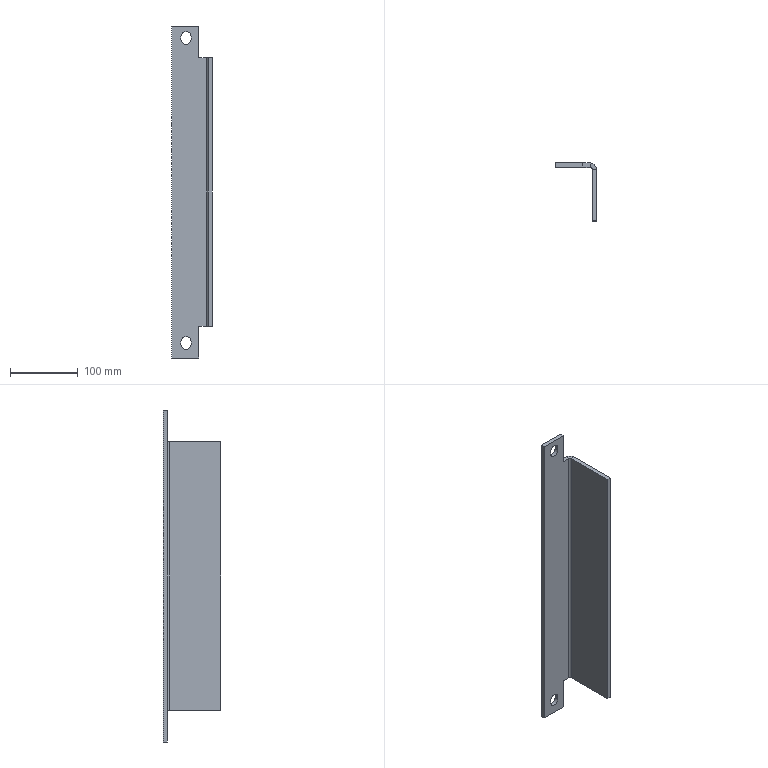Part | SolidWorks | features ICE 2, FlatPattern 1, SMBaseFlange 1, SheetMetal 1 | 1 solid | 28 faces | box 60 x 85 x 490 mm | volume 343865 mm3 | plane 20 | cylinder 8 | commonest cylinder face diameters 15 x6 6 x1 18 x1
STEP:
#1=CARTESIAN_POINT('',(-38.8,-6.,-213.5));
#2=VERTEX_POINT('',#1);
#3=CARTESIAN_POINT('',(-31.3,-6.,-221.));
#4=VERTEX_POINT('',#3);
#5=CARTESIAN_POINT('',(-38.8,-6.,-221.));
#6=DIRECTION('',(0.,1.,0.));
#7=DIRECTION('',(-1.,0.,0.));
#8=AXIS2_PLACEMENT_3D('',#5,#6,#7);
#9=CIRCLE('',#8,7.5);
#10=EDGE_CURVE('',#2,#4,#9,.T.);
#11=ORIENTED_EDGE('',*,*,#10,.F.);
#12=CARTESIAN_POINT('',(-38.8,0.,-213.5));
#13=VERTEX_POINT('',#12);
#14=CARTESIAN_POINT('',(-38.8,-85.,-213.5));
#15=DIRECTION('',(0.,1.,0.));
#16=VECTOR('',#15,1000.);
#17=LINE('',#14,#16);
#18=EDGE_CURVE('',#2,#13,#17,.T.);
#19=ORIENTED_EDGE('',*,*,#18,.T.);
#20=CARTESIAN_POINT('',(-31.3,0.,-221.));
#21=VERTEX_POINT('',#20);
#22=CARTESIAN_POINT('',(-38.8,0.,-221.));
#23=DIRECTION('',(0.,1.,0.));
#24=DIRECTION('',(0.,0.,1.));
#25=AXIS2_PLACEMENT_3D('',#22,#23,#24);
#26=CIRCLE('',#25,7.5);
#27=EDGE_CURVE('',#13,#21,#26,.T.);
#28=ORIENTED_EDGE('',*,*,#27,.T.);
#29=CARTESIAN_POINT('',(-31.3,-85.,-221.));
#30=DIRECTION('',(0.,1.,0.));
#31=VECTOR('',#30,1000.);
#32=LINE('',#29,#31);
#33=EDGE_CURVE('',#4,#21,#32,.T.);
#34=ORIENTED_EDGE('',*,*,#33,.F.);
#35=EDGE_LOOP('',(#11,#19,#28,#34));
#36=FACE_OUTER_BOUND('',#35,.T.);
#37=CARTESIAN_POINT('',(-38.8,-85.,-221.));
#38=DIRECTION('',(0.,1.,0.));
#39=DIRECTION('',(0.,0.,1.));
#40=AXIS2_PLACEMENT_3D('',#37,#38,#39);
#41=CYLINDRICAL_SURFACE('',#40,7.5);
#42=ADVANCED_FACE('',(#36),#41,.F.);
#43=CARTESIAN_POINT('',(-38.8,-6.,236.5));
#44=VERTEX_POINT('',#43);
#45=CARTESIAN_POINT('',(-31.3,-6.,229.));
#46=VERTEX_POINT('',#45);
#47=CARTESIAN_POINT('',(-38.8,-6.,229.));
#48=DIRECTION('',(0.,1.,0.));
#49=DIRECTION('',(-1.,0.,0.));
#50=AXIS2_PLACEMENT_3D('',#47,#48,#49);
#51=CIRCLE('',#50,7.5);
#52=EDGE_CURVE('',#44,#46,#51,.T.);
#53=ORIENTED_EDGE('',*,*,#52,.F.);
#54=CARTESIAN_POINT('',(-38.8,0.,236.5));
#55=VERTEX_POINT('',#54);
#56=CARTESIAN_POINT('',(-38.8,-85.,236.5));
#57=DIRECTION('',(0.,1.,0.));
#58=VECTOR('',#57,1000.);
#59=LINE('',#56,#58);
#60=EDGE_CURVE('',#44,#55,#59,.T.);
#61=ORIENTED_EDGE('',*,*,#60,.T.);
#62=CARTESIAN_POINT('',(-31.3,0.,229.));
#63=VERTEX_POINT('',#62);
#64=CARTESIAN_POINT('',(-38.8,0.,229.));
#65=DIRECTION('',(0.,1.,0.));
#66=DIRECTION('',(0.,0.,1.));
#67=AXIS2_PLACEMENT_3D('',#64,#65,#66);
#68=CIRCLE('',#67,7.5);
#69=EDGE_CURVE('',#55,#63,#68,.T.);
#70=ORIENTED_EDGE('',*,*,#69,.T.);
#71=CARTESIAN_POINT('',(-31.3,-85.,229.));
#72=DIRECTION('',(0.,1.,0.));
#73=VECTOR('',#72,1000.);
#74=LINE('',#71,#73);
#75=EDGE_CURVE('',#46,#63,#74,.T.);
#76=ORIENTED_EDGE('',*,*,#75,.F.);
#77=EDGE_LOOP('',(#53,#61,#70,#76));
#78=FACE_OUTER_BOUND('',#77,.T.);
#79=CARTESIAN_POINT('',(-38.8,-85.,229.));
#80=DIRECTION('',(0.,1.,0.));
#81=DIRECTION('',(0.,0.,1.));
#82=AXIS2_PLACEMENT_3D('',#79,#80,#81);
#83=CYLINDRICAL_SURFACE('',#82,7.5);
#84=ADVANCED_FACE('',(#78),#83,.F.);
#85=CARTESIAN_POINT('',(-6.,-9.,-198.));
#86=VERTEX_POINT('',#85);
#87=CARTESIAN_POINT('',(-6.,-85.,-198.));
#88=VERTEX_POINT('',#87);
#89=CARTESIAN_POINT('',(-6.,0.,-198.));
#90=DIRECTION('',(0.,-1.,0.));
#91=VECTOR('',#90,1000.);
#92=LINE('',#89,#91);
#93=EDGE_CURVE('',#86,#88,#92,.T.);
#94=ORIENTED_EDGE('',*,*,#93,.F.);
#95=CARTESIAN_POINT('',(0.,-9.,-198.));
#96=VERTEX_POINT('',#95);
#97=CARTESIAN_POINT('',(-6.,-9.,-198.));
#98=DIRECTION('',(1.,0.,0.));
#99=VECTOR('',#98,1000.);
#100=LINE('',#97,#99);
#101=EDGE_CURVE('',#86,#96,#100,.T.);
#102=ORIENTED_EDGE('',*,*,#101,.T.);
#103=CARTESIAN_POINT('',(0.,-85.,-198.));
#104=VERTEX_POINT('',#103);
#105=CARTESIAN_POINT('',(0.,-85.,-198.));
#106=DIRECTION('',(0.,-1.,0.));
#107=VECTOR('',#106,1000.);
#108=LINE('',#105,#107);
#109=EDGE_CURVE('',#96,#104,#108,.T.);
#110=ORIENTED_EDGE('',*,*,#109,.T.);
#111=CARTESIAN_POINT('',(-20.,-85.,-198.));
#112=DIRECTION('',(1.,0.,0.));
#113=VECTOR('',#112,1000.);
#114=LINE('',#111,#113);
#115=EDGE_CURVE('',#88,#104,#114,.T.);
#116=ORIENTED_EDGE('',*,*,#115,.F.);
#117=EDGE_LOOP('',(#94,#102,#110,#116));
#118=FACE_OUTER_BOUND('',#117,.T.);
#119=CARTESIAN_POINT('',(-20.,-85.,-198.));
#120=DIRECTION('',(0.,0.,1.));
#121=DIRECTION('',(1.,0.,0.));
#122=AXIS2_PLACEMENT_3D('',#119,#120,#121);
#123=PLANE('',#122);
#124=ADVANCED_FACE('',(#118),#123,.F.);
#125=CARTESIAN_POINT('',(-20.,0.,-198.));
#126=VERTEX_POINT('',#125);
#127=CARTESIAN_POINT('',(-9.,0.,-198.));
#128=VERTEX_POINT('',#127);
#129=CARTESIAN_POINT('',(-20.,0.,-198.));
#130=DIRECTION('',(1.,0.,0.));
#131=VECTOR('',#130,1000.);
#132=LINE('',#129,#131);
#133=EDGE_CURVE('',#126,#128,#132,.T.);
#134=ORIENTED_EDGE('',*,*,#133,.T.);
#135=CARTESIAN_POINT('',(-9.,-6.,-198.));
#136=VERTEX_POINT('',#135);
#137=CARTESIAN_POINT('',(-9.,0.,-198.));
#138=DIRECTION('',(0.,-1.,0.));
#139=VECTOR('',#138,1000.);
#140=LINE('',#137,#139);
#141=EDGE_CURVE('',#128,#136,#140,.T.);
#142=ORIENTED_EDGE('',*,*,#141,.T.);
#143=CARTESIAN_POINT('',(-20.,-6.,-198.));
#144=VERTEX_POINT('',#143);
#145=CARTESIAN_POINT('',(0.,-6.,-198.));
#146=DIRECTION('',(1.,0.,0.));
#147=VECTOR('',#146,1000.);
#148=LINE('',#145,#147);
#149=EDGE_CURVE('',#144,#136,#148,.T.);
#150=ORIENTED_EDGE('',*,*,#149,.F.);
#151=CARTESIAN_POINT('',(-20.,-85.,-198.));
#152=DIRECTION('',(0.,-1.,0.));
#153=VECTOR('',#152,1000.);
#154=LINE('',#151,#153);
#155=EDGE_CURVE('',#126,#144,#154,.T.);
#156=ORIENTED_EDGE('',*,*,#155,.F.);
#157=EDGE_LOOP('',(#134,#142,#150,#156));
#158=FACE_OUTER_BOUND('',#157,.T.);
#159=CARTESIAN_POINT('',(-20.,-85.,-198.));
#160=DIRECTION('',(0.,0.,1.));
#161=DIRECTION('',(1.,0.,0.));
#162=AXIS2_PLACEMENT_3D('',#159,#160,#161);
#163=PLANE('',#162);
#164=ADVANCED_FACE('',(#158),#163,.F.);
#165=CARTESIAN_POINT('',(-9.,-6.,198.));
#166=VERTEX_POINT('',#165);
#167=CARTESIAN_POINT('',(-20.,-6.,198.));
#168=VERTEX_POINT('',#167);
#169=CARTESIAN_POINT('',(0.,-6.,198.));
#170=DIRECTION('',(-1.,0.,0.));
#171=VECTOR('',#170,1000.);
#172=LINE('',#169,#171);
#173=EDGE_CURVE('',#166,#168,#172,.T.);
#174=ORIENTED_EDGE('',*,*,#173,.F.);
#175=CARTESIAN_POINT('',(-9.,0.,198.));
#176=VERTEX_POINT('',#175);
#177=CARTESIAN_POINT('',(-9.,-6.,198.));
#178=DIRECTION('',(0.,1.,0.));
#179=VECTOR('',#178,1000.);
#180=LINE('',#177,#179);
#181=EDGE_CURVE('',#166,#176,#180,.T.);
#182=ORIENTED_EDGE('',*,*,#181,.T.);
#183=CARTESIAN_POINT('',(-20.,0.,198.));
#184=VERTEX_POINT('',#183);
#185=CARTESIAN_POINT('',(-20.,0.,198.));
#186=DIRECTION('',(1.,0.,0.));
#187=VECTOR('',#186,1000.);
#188=LINE('',#185,#187);
#189=EDGE_CURVE('',#184,#176,#188,.T.);
#190=ORIENTED_EDGE('',*,*,#189,.F.);
#191=CARTESIAN_POINT('',(-20.,-85.,198.));
#192=DIRECTION('',(0.,1.,0.));
#193=VECTOR('',#192,1000.);
#194=LINE('',#191,#193);
#195=EDGE_CURVE('',#168,#184,#194,.T.);
#196=ORIENTED_EDGE('',*,*,#195,.F.);
#197=EDGE_LOOP('',(#174,#182,#190,#196));
#198=FACE_OUTER_BOUND('',#197,.T.);
#199=CARTESIAN_POINT('',(-20.,-85.,198.));
#200=DIRECTION('',(0.,0.,-1.));
#201=DIRECTION('',(-1.,0.,0.));
#202=AXIS2_PLACEMENT_3D('',#199,#200,#201);
#203=PLANE('',#202);
#204=ADVANCED_FACE('',(#198),#203,.F.);
#205=CARTESIAN_POINT('',(0.,-85.,198.));
#206=VERTEX_POINT('',#205);
#207=CARTESIAN_POINT('',(0.,-9.,198.));
#208=VERTEX_POINT('',#207);
#209=CARTESIAN_POINT('',(0.,-85.,198.));
#210=DIRECTION('',(0.,1.,0.));
#211=VECTOR('',#210,1000.);
#212=LINE('',#209,#211);
#213=EDGE_CURVE('',#206,#208,#212,.T.);
#214=ORIENTED_EDGE('',*,*,#213,.T.);
#215=CARTESIAN_POINT('',(-6.,-9.,198.));
#216=VERTEX_POINT('',#215);
#217=CARTESIAN_POINT('',(0.,-9.,198.));
#218=DIRECTION('',(-1.,0.,0.));
#219=VECTOR('',#218,1000.);
#220=LINE('',#217,#219);
#221=EDGE_CURVE('',#208,#216,#220,.T.);
#222=ORIENTED_EDGE('',*,*,#221,.T.);
#223=CARTESIAN_POINT('',(-6.,-85.,198.));
#224=VERTEX_POINT('',#223);
#225=CARTESIAN_POINT('',(-6.,0.,198.));
#226=DIRECTION('',(0.,1.,0.));
#227=VECTOR('',#226,1000.);
#228=LINE('',#225,#227);
#229=EDGE_CURVE('',#224,#216,#228,.T.);
#230=ORIENTED_EDGE('',*,*,#229,.F.);
#231=CARTESIAN_POINT('',(-20.,-85.,198.));
#232=DIRECTION('',(1.,0.,0.));
#233=VECTOR('',#232,1000.);
#234=LINE('',#231,#233);
#235=EDGE_CURVE('',#224,#206,#234,.T.);
#236=ORIENTED_EDGE('',*,*,#235,.T.);
#237=EDGE_LOOP('',(#214,#222,#230,#236));
#238=FACE_OUTER_BOUND('',#237,.T.);
#239=CARTESIAN_POINT('',(-20.,-85.,198.));
#240=DIRECTION('',(0.,0.,-1.));
#241=DIRECTION('',(-1.,0.,0.));
#242=AXIS2_PLACEMENT_3D('',#239,#240,#241);
#243=PLANE('',#242);
#244=ADVANCED_FACE('',(#238),#243,.F.);
#245=CARTESIAN_POINT('',(-20.,-6.,-245.));
#246=VERTEX_POINT('',#245);
#247=CARTESIAN_POINT('',(-20.,0.,-245.));
#248=VERTEX_POINT('',#247);
#249=CARTESIAN_POINT('',(-20.,-85.,-245.));
#250=DIRECTION('',(0.,1.,0.));
#251=VECTOR('',#250,1000.);
#252=LINE('',#249,#251);
#253=EDGE_CURVE('',#246,#248,#252,.T.);
#254=ORIENTED_EDGE('',*,*,#253,.F.);
#255=CARTESIAN_POINT('',(-60.,-6.,-245.));
#256=VERTEX_POINT('',#255);
#257=CARTESIAN_POINT('',(0.,-6.,-245.));
#258=DIRECTION('',(1.,0.,0.));
#259=VECTOR('',#258,1000.);
#260=LINE('',#257,#259);
#261=EDGE_CURVE('',#256,#246,#260,.T.);
#262=ORIENTED_EDGE('',*,*,#261,.F.);
#263=CARTESIAN_POINT('',(-60.,0.,-245.));
#264=VERTEX_POINT('',#263);
#265=CARTESIAN_POINT('',(-60.,-6.,-245.));
#266=DIRECTION('',(0.,1.,0.));
#267=VECTOR('',#266,1000.);
#268=LINE('',#265,#267);
#269=EDGE_CURVE('',#256,#264,#268,.T.);
#270=ORIENTED_EDGE('',*,*,#269,.T.);
#271=CARTESIAN_POINT('',(0.,0.,-245.));
#272=DIRECTION('',(1.,0.,0.));
#273=VECTOR('',#272,1000.);
#274=LINE('',#271,#273);
#275=EDGE_CURVE('',#264,#248,#274,.T.);
#276=ORIENTED_EDGE('',*,*,#275,.T.);
#277=EDGE_LOOP('',(#254,#262,#270,#276));
#278=FACE_OUTER_BOUND('',#277,.T.);
#279=CARTESIAN_POINT('',(-6.,-9.,-245.));
#280=DIRECTION('',(0.,0.,-1.));
#281=DIRECTION('',(-1.,0.,0.));
#282=AXIS2_PLACEMENT_3D('',#279,#280,#281);
#283=PLANE('',#282);
#284=ADVANCED_FACE('',(#278),#283,.T.);
#285=CARTESIAN_POINT('',(-6.,-85.,245.));
#286=DIRECTION('',(0.,0.,-1.));
#287=VECTOR('',#286,1000.);
#288=LINE('',#285,#287);
#289=EDGE_CURVE('',#224,#88,#288,.T.);
#290=ORIENTED_EDGE('',*,*,#289,.F.);
#291=ORIENTED_EDGE('',*,*,#229,.T.);
#292=CARTESIAN_POINT('',(-6.,-9.,245.));
#293=DIRECTION('',(0.,0.,-1.));
#294=VECTOR('',#293,1000.);
#295=LINE('',#292,#294);
#296=EDGE_CURVE('',#216,#86,#295,.T.);
#297=ORIENTED_EDGE('',*,*,#296,.T.);
#298=ORIENTED_EDGE('',*,*,#93,.T.);
#299=EDGE_LOOP('',(#290,#291,#297,#298));
#300=FACE_OUTER_BOUND('',#299,.T.);
#301=CARTESIAN_POINT('',(-6.,0.,245.));
#302=DIRECTION('',(1.,0.,0.));
#303=DIRECTION('',(0.,1.,0.));
#304=AXIS2_PLACEMENT_3D('',#301,#302,#303);
#305=PLANE('',#304);
#306=ADVANCED_FACE('',(#300),#305,.F.);
#307=ORIENTED_EDGE('',*,*,#235,.F.);
#308=ORIENTED_EDGE('',*,*,#289,.T.);
#309=ORIENTED_EDGE('',*,*,#115,.T.);
#310=CARTESIAN_POINT('',(0.,-85.,245.));
#311=DIRECTION('',(0.,0.,-1.));
#312=VECTOR('',#311,1000.);
#313=LINE('',#310,#312);
#314=EDGE_CURVE('',#206,#104,#313,.T.);
#315=ORIENTED_EDGE('',*,*,#314,.F.);
#316=EDGE_LOOP('',(#307,#308,#309,#315));
#317=FACE_OUTER_BOUND('',#316,.T.);
#318=CARTESIAN_POINT('',(0.,-85.,245.));
#319=DIRECTION('',(0.,-1.,0.));
#320=DIRECTION('',(0.,0.,-1.));
#321=AXIS2_PLACEMENT_3D('',#318,#319,#320);
#322=PLANE('',#321);
#323=ADVANCED_FACE('',(#317),#322,.T.);
#324=ORIENTED_EDGE('',*,*,#213,.F.);
#325=ORIENTED_EDGE('',*,*,#314,.T.);
#326=ORIENTED_EDGE('',*,*,#109,.F.);
#327=CARTESIAN_POINT('',(0.,-9.,245.));
#328=DIRECTION('',(0.,0.,-1.));
#329=VECTOR('',#328,1000.);
#330=LINE('',#327,#329);
#331=EDGE_CURVE('',#208,#96,#330,.T.);
#332=ORIENTED_EDGE('',*,*,#331,.F.);
#333=EDGE_LOOP('',(#324,#325,#326,#332));
#334=FACE_OUTER_BOUND('',#333,.T.);
#335=CARTESIAN_POINT('',(0.,0.,245.));
#336=DIRECTION('',(1.,0.,0.));
#337=DIRECTION('',(0.,1.,0.));
#338=AXIS2_PLACEMENT_3D('',#335,#336,#337);
#339=PLANE('',#338);
#340=ADVANCED_FACE('',(#334),#339,.T.);
#341=CARTESIAN_POINT('',(-9.,-9.,198.));
#342=DIRECTION('',(0.,0.,1.));
#343=DIRECTION('',(-1.,0.,0.));
#344=AXIS2_PLACEMENT_3D('',#341,#342,#343);
#345=CIRCLE('',#344,9.);
#346=EDGE_CURVE('',#208,#176,#345,.T.);
#347=ORIENTED_EDGE('',*,*,#346,.F.);
#348=ORIENTED_EDGE('',*,*,#331,.T.);
#349=CARTESIAN_POINT('',(-9.,-9.,-198.));
#350=DIRECTION('',(0.,0.,-1.));
#351=DIRECTION('',(1.,0.,0.));
#352=AXIS2_PLACEMENT_3D('',#349,#350,#351);
#353=CIRCLE('',#352,9.);
#354=EDGE_CURVE('',#128,#96,#353,.T.);
#355=ORIENTED_EDGE('',*,*,#354,.F.);
#356=CARTESIAN_POINT('',(-9.,0.,245.));
#357=DIRECTION('',(0.,0.,-1.));
#358=VECTOR('',#357,1000.);
#359=LINE('',#356,#358);
#360=EDGE_CURVE('',#176,#128,#359,.T.);
#361=ORIENTED_EDGE('',*,*,#360,.F.);
#362=EDGE_LOOP('',(#347,#348,#355,#361));
#363=FACE_OUTER_BOUND('',#362,.T.);
#364=CARTESIAN_POINT('',(-9.,-9.,245.));
#365=DIRECTION('',(0.,0.,-1.));
#366=DIRECTION('',(-1.,0.,0.));
#367=AXIS2_PLACEMENT_3D('',#364,#365,#366);
#368=CYLINDRICAL_SURFACE('',#367,9.);
#369=ADVANCED_FACE('',(#363),#368,.T.);
#370=ORIENTED_EDGE('',*,*,#189,.T.);
#371=ORIENTED_EDGE('',*,*,#360,.T.);
#372=ORIENTED_EDGE('',*,*,#133,.F.);
#373=CARTESIAN_POINT('',(-20.,0.,-245.));
#374=DIRECTION('',(0.,0.,1.));
#375=VECTOR('',#374,1000.);
#376=LINE('',#373,#375);
#377=EDGE_CURVE('',#248,#126,#376,.T.);
#378=ORIENTED_EDGE('',*,*,#377,.F.);
#379=ORIENTED_EDGE('',*,*,#275,.F.);
#380=CARTESIAN_POINT('',(-60.,0.,245.));
#381=VERTEX_POINT('',#380);
#382=CARTESIAN_POINT('',(-60.,0.,245.));
#383=DIRECTION('',(0.,0.,-1.));
#384=VECTOR('',#383,1000.);
#385=LINE('',#382,#384);
#386=EDGE_CURVE('',#381,#264,#385,.T.);
#387=ORIENTED_EDGE('',*,*,#386,.F.);
#388=CARTESIAN_POINT('',(-20.,0.,245.));
#389=VERTEX_POINT('',#388);
#390=CARTESIAN_POINT('',(0.,0.,245.));
#391=DIRECTION('',(1.,0.,0.));
#392=VECTOR('',#391,1000.);
#393=LINE('',#390,#392);
#394=EDGE_CURVE('',#381,#389,#393,.T.);
#395=ORIENTED_EDGE('',*,*,#394,.T.);
#396=CARTESIAN_POINT('',(-20.,0.,245.));
#397=DIRECTION('',(0.,0.,1.));
#398=VECTOR('',#397,1000.);
#399=LINE('',#396,#398);
#400=EDGE_CURVE('',#184,#389,#399,.T.);
#401=ORIENTED_EDGE('',*,*,#400,.F.);
#402=EDGE_LOOP('',(#370,#371,#372,#378,#379,#387,#395,#401));
#403=FACE_OUTER_BOUND('',#402,.T.);
#404=CARTESIAN_POINT('',(-31.3,0.,-225.));
#405=VERTEX_POINT('',#404);
#406=CARTESIAN_POINT('',(-46.3,0.,-225.));
#407=VERTEX_POINT('',#406);
#408=CARTESIAN_POINT('',(-38.8,0.,-225.));
#409=DIRECTION('',(0.,1.,0.));
#410=DIRECTION('',(0.,0.,1.));
#411=AXIS2_PLACEMENT_3D('',#408,#409,#410);
#412=CIRCLE('',#411,7.5);
#413=EDGE_CURVE('',#405,#407,#412,.T.);
#414=ORIENTED_EDGE('',*,*,#413,.F.);
#415=CARTESIAN_POINT('',(-31.3,0.,-225.));
#416=DIRECTION('',(0.,0.,-1.));
#417=VECTOR('',#416,1000.);
#418=LINE('',#415,#417);
#419=EDGE_CURVE('',#21,#405,#418,.T.);
#420=ORIENTED_EDGE('',*,*,#419,.F.);
#421=ORIENTED_EDGE('',*,*,#27,.F.);
#422=CARTESIAN_POINT('',(-46.3,0.,-221.));
#423=VERTEX_POINT('',#422);
#424=CARTESIAN_POINT('',(-38.8,0.,-221.));
#425=DIRECTION('',(0.,1.,0.));
#426=DIRECTION('',(0.,0.,1.));
#427=AXIS2_PLACEMENT_3D('',#424,#425,#426);
#428=CIRCLE('',#427,7.5);
#429=EDGE_CURVE('',#423,#13,#428,.T.);
#430=ORIENTED_EDGE('',*,*,#429,.F.);
#431=CARTESIAN_POINT('',(-46.3,0.,-225.));
#432=DIRECTION('',(0.,0.,1.));
#433=VECTOR('',#432,1000.);
#434=LINE('',#431,#433);
#435=EDGE_CURVE('',#407,#423,#434,.T.);
#436=ORIENTED_EDGE('',*,*,#435,.F.);
#437=EDGE_LOOP('',(#414,#420,#421,#430,#436));
#438=FACE_BOUND('',#437,.T.);
#439=CARTESIAN_POINT('',(-31.3,0.,225.));
#440=VERTEX_POINT('',#439);
#441=CARTESIAN_POINT('',(-46.3,0.,225.));
#442=VERTEX_POINT('',#441);
#443=CARTESIAN_POINT('',(-38.8,0.,225.));
#444=DIRECTION('',(0.,1.,0.));
#445=DIRECTION('',(0.,0.,1.));
#446=AXIS2_PLACEMENT_3D('',#443,#444,#445);
#447=CIRCLE('',#446,7.5);
#448=EDGE_CURVE('',#440,#442,#447,.T.);
#449=ORIENTED_EDGE('',*,*,#448,.F.);
#450=CARTESIAN_POINT('',(-31.3,0.,225.));
#451=DIRECTION('',(0.,0.,-1.));
#452=VECTOR('',#451,1000.);
#453=LINE('',#450,#452);
#454=EDGE_CURVE('',#63,#440,#453,.T.);
#455=ORIENTED_EDGE('',*,*,#454,.F.);
#456=ORIENTED_EDGE('',*,*,#69,.F.);
#457=CARTESIAN_POINT('',(-46.3,0.,229.));
#458=VERTEX_POINT('',#457);
#459=CARTESIAN_POINT('',(-38.8,0.,229.));
#460=DIRECTION('',(0.,1.,0.));
#461=DIRECTION('',(0.,0.,1.));
#462=AXIS2_PLACEMENT_3D('',#459,#460,#461);
#463=CIRCLE('',#462,7.5);
#464=EDGE_CURVE('',#458,#55,#463,.T.);
#465=ORIENTED_EDGE('',*,*,#464,.F.);
#466=CARTESIAN_POINT('',(-46.3,0.,225.));
#467=DIRECTION('',(0.,0.,1.));
#468=VECTOR('',#467,1000.);
#469=LINE('',#466,#468);
#470=EDGE_CURVE('',#442,#458,#469,.T.);
#471=ORIENTED_EDGE('',*,*,#470,.F.);
#472=EDGE_LOOP('',(#449,#455,#456,#465,#471));
#473=FACE_BOUND('',#472,.T.);
#474=CARTESIAN_POINT('',(0.,0.,245.));
#475=DIRECTION('',(0.,1.,0.));
#476=DIRECTION('',(-1.,0.,0.));
#477=AXIS2_PLACEMENT_3D('',#474,#475,#476);
#478=PLANE('',#477);
#479=ADVANCED_FACE('',(#403,#438,#473),#478,.T.);
#480=ORIENTED_EDGE('',*,*,#269,.F.);
#481=CARTESIAN_POINT('',(-60.,-6.,245.));
#482=VERTEX_POINT('',#481);
#483=CARTESIAN_POINT('',(-60.,-6.,245.));
#484=DIRECTION('',(0.,0.,-1.));
#485=VECTOR('',#484,1000.);
#486=LINE('',#483,#485);
#487=EDGE_CURVE('',#482,#256,#486,.T.);
#488=ORIENTED_EDGE('',*,*,#487,.F.);
#489=CARTESIAN_POINT('',(-60.,-6.,245.));
#490=DIRECTION('',(0.,1.,0.));
#491=VECTOR('',#490,1000.);
#492=LINE('',#489,#491);
#493=EDGE_CURVE('',#482,#381,#492,.T.);
#494=ORIENTED_EDGE('',*,*,#493,.T.);
#495=ORIENTED_EDGE('',*,*,#386,.T.);
#496=EDGE_LOOP('',(#480,#488,#494,#495));
#497=FACE_OUTER_BOUND('',#496,.T.);
#498=CARTESIAN_POINT('',(-60.,-6.,245.));
#499=DIRECTION('',(-1.,0.,0.));
#500=DIRECTION('',(0.,0.,1.));
#501=AXIS2_PLACEMENT_3D('',#498,#499,#500);
#502=PLANE('',#501);
#503=ADVANCED_FACE('',(#497),#502,.T.);
#504=CARTESIAN_POINT('',(-31.3,-6.,-225.));
#505=VERTEX_POINT('',#504);
#506=CARTESIAN_POINT('',(-31.3,-6.,245.));
#507=DIRECTION('',(0.,0.,-1.));
#508=VECTOR('',#507,1000.);
#509=LINE('',#506,#508);
#510=EDGE_CURVE('',#4,#505,#509,.T.);
#511=ORIENTED_EDGE('',*,*,#510,.T.);
#512=CARTESIAN_POINT('',(-46.3,-6.,-225.));
#513=VERTEX_POINT('',#512);
#514=CARTESIAN_POINT('',(-38.8,-6.,-225.));
#515=DIRECTION('',(0.,1.,0.));
#516=DIRECTION('',(-1.,0.,0.));
#517=AXIS2_PLACEMENT_3D('',#514,#515,#516);
#518=CIRCLE('',#517,7.5);
#519=EDGE_CURVE('',#505,#513,#518,.T.);
#520=ORIENTED_EDGE('',*,*,#519,.T.);
#521=CARTESIAN_POINT('',(-46.3,-6.,-221.));
#522=VERTEX_POINT('',#521);
#523=CARTESIAN_POINT('',(-46.3,-6.,245.));
#524=DIRECTION('',(0.,0.,1.));
#525=VECTOR('',#524,1000.);
#526=LINE('',#523,#525);
#527=EDGE_CURVE('',#513,#522,#526,.T.);
#528=ORIENTED_EDGE('',*,*,#527,.T.);
#529=CARTESIAN_POINT('',(-38.8,-6.,-221.));
#530=DIRECTION('',(0.,1.,0.));
#531=DIRECTION('',(-1.,0.,0.));
#532=AXIS2_PLACEMENT_3D('',#529,#530,#531);
#533=CIRCLE('',#532,7.5);
#534=EDGE_CURVE('',#522,#2,#533,.T.);
#535=ORIENTED_EDGE('',*,*,#534,.T.);
#536=ORIENTED_EDGE('',*,*,#10,.T.);
#537=EDGE_LOOP('',(#511,#520,#528,#535,#536));
#538=FACE_BOUND('',#537,.T.);
#539=CARTESIAN_POINT('',(-31.3,-6.,225.));
#540=VERTEX_POINT('',#539);
#541=CARTESIAN_POINT('',(-31.3,-6.,245.));
#542=DIRECTION('',(0.,0.,-1.));
#543=VECTOR('',#542,1000.);
#544=LINE('',#541,#543);
#545=EDGE_CURVE('',#46,#540,#544,.T.);
#546=ORIENTED_EDGE('',*,*,#545,.T.);
#547=CARTESIAN_POINT('',(-46.3,-6.,225.));
#548=VERTEX_POINT('',#547);
#549=CARTESIAN_POINT('',(-38.8,-6.,225.));
#550=DIRECTION('',(0.,1.,0.));
#551=DIRECTION('',(-1.,0.,0.));
#552=AXIS2_PLACEMENT_3D('',#549,#550,#551);
#553=CIRCLE('',#552,7.5);
#554=EDGE_CURVE('',#540,#548,#553,.T.);
#555=ORIENTED_EDGE('',*,*,#554,.T.);
#556=CARTESIAN_POINT('',(-46.3,-6.,229.));
#557=VERTEX_POINT('',#556);
#558=CARTESIAN_POINT('',(-46.3,-6.,245.));
#559=DIRECTION('',(0.,0.,1.));
#560=VECTOR('',#559,1000.);
#561=LINE('',#558,#560);
#562=EDGE_CURVE('',#548,#557,#561,.T.);
#563=ORIENTED_EDGE('',*,*,#562,.T.);
#564=CARTESIAN_POINT('',(-38.8,-6.,229.));
#565=DIRECTION('',(0.,1.,0.));
#566=DIRECTION('',(-1.,0.,0.));
#567=AXIS2_PLACEMENT_3D('',#564,#565,#566);
#568=CIRCLE('',#567,7.5);
#569=EDGE_CURVE('',#557,#44,#568,.T.);
#570=ORIENTED_EDGE('',*,*,#569,.T.);
#571=ORIENTED_EDGE('',*,*,#52,.T.);
#572=EDGE_LOOP('',(#546,#555,#563,#570,#571));
#573=FACE_BOUND('',#572,.T.);
#574=CARTESIAN_POINT('',(-9.,-6.,245.));
#575=DIRECTION('',(0.,0.,-1.));
#576=VECTOR('',#575,1000.);
#577=LINE('',#574,#576);
#578=EDGE_CURVE('',#166,#136,#577,.T.);
#579=ORIENTED_EDGE('',*,*,#578,.F.);
#580=ORIENTED_EDGE('',*,*,#173,.T.);
#581=CARTESIAN_POINT('',(-20.,-6.,245.));
#582=VERTEX_POINT('',#581);
#583=CARTESIAN_POINT('',(-20.,-6.,245.));
#584=DIRECTION('',(0.,0.,1.));
#585=VECTOR('',#584,1000.);
#586=LINE('',#583,#585);
#587=EDGE_CURVE('',#168,#582,#586,.T.);
#588=ORIENTED_EDGE('',*,*,#587,.T.);
#589=CARTESIAN_POINT('',(0.,-6.,245.));
#590=DIRECTION('',(1.,0.,0.));
#591=VECTOR('',#590,1000.);
#592=LINE('',#589,#591);
#593=EDGE_CURVE('',#482,#582,#592,.T.);
#594=ORIENTED_EDGE('',*,*,#593,.F.);
#595=ORIENTED_EDGE('',*,*,#487,.T.);
#596=ORIENTED_EDGE('',*,*,#261,.T.);
#597=CARTESIAN_POINT('',(-20.,-6.,245.));
#598=DIRECTION('',(0.,0.,1.));
#599=VECTOR('',#598,1000.);
#600=LINE('',#597,#599);
#601=EDGE_CURVE('',#246,#144,#600,.T.);
#602=ORIENTED_EDGE('',*,*,#601,.T.);
#603=ORIENTED_EDGE('',*,*,#149,.T.);
#604=EDGE_LOOP('',(#579,#580,#588,#594,#595,#596,#602,#603));
#605=FACE_OUTER_BOUND('',#604,.T.);
#606=CARTESIAN_POINT('',(0.,-6.,245.));
#607=DIRECTION('',(0.,1.,0.));
#608=DIRECTION('',(-1.,0.,0.));
#609=AXIS2_PLACEMENT_3D('',#606,#607,#608);
#610=PLANE('',#609);
#611=ADVANCED_FACE('',(#538,#573,#605),#610,.F.);
#612=ORIENTED_EDGE('',*,*,#296,.F.);
#613=CARTESIAN_POINT('',(-9.,-9.,198.));
#614=DIRECTION('',(0.,0.,1.));
#615=DIRECTION('',(-1.,0.,0.));
#616=AXIS2_PLACEMENT_3D('',#613,#614,#615);
#617=CIRCLE('',#616,3.);
#618=EDGE_CURVE('',#216,#166,#617,.T.);
#619=ORIENTED_EDGE('',*,*,#618,.T.);
#620=ORIENTED_EDGE('',*,*,#578,.T.);
#621=CARTESIAN_POINT('',(-9.,-9.,-198.));
#622=DIRECTION('',(0.,0.,-1.));
#623=DIRECTION('',(1.,0.,0.));
#624=AXIS2_PLACEMENT_3D('',#621,#622,#623);
#625=CIRCLE('',#624,3.);
#626=EDGE_CURVE('',#136,#86,#625,.T.);
#627=ORIENTED_EDGE('',*,*,#626,.T.);
#628=EDGE_LOOP('',(#612,#619,#620,#627));
#629=FACE_OUTER_BOUND('',#628,.T.);
#630=CARTESIAN_POINT('',(-9.,-9.,245.));
#631=DIRECTION('',(0.,0.,-1.));
#632=DIRECTION('',(-1.,0.,0.));
#633=AXIS2_PLACEMENT_3D('',#630,#631,#632);
#634=CYLINDRICAL_SURFACE('',#633,3.);
#635=ADVANCED_FACE('',(#629),#634,.F.);
#636=CARTESIAN_POINT('',(-20.,-85.,245.));
#637=DIRECTION('',(0.,-1.,0.));
#638=VECTOR('',#637,1000.);
#639=LINE('',#636,#638);
#640=EDGE_CURVE('',#389,#582,#639,.T.);
#641=ORIENTED_EDGE('',*,*,#640,.F.);
#642=ORIENTED_EDGE('',*,*,#394,.F.);
#643=ORIENTED_EDGE('',*,*,#493,.F.);
#644=ORIENTED_EDGE('',*,*,#593,.T.);
#645=EDGE_LOOP('',(#641,#642,#643,#644));
#646=FACE_OUTER_BOUND('',#645,.T.);
#647=CARTESIAN_POINT('',(-9.,-9.,245.));
#648=DIRECTION('',(0.,0.,1.));
#649=DIRECTION('',(1.,0.,0.));
#650=AXIS2_PLACEMENT_3D('',#647,#648,#649);
#651=PLANE('',#650);
#652=ADVANCED_FACE('',(#646),#651,.T.);
#653=CARTESIAN_POINT('',(-31.3,-85.,225.));
#654=DIRECTION('',(0.,1.,0.));
#655=VECTOR('',#654,1000.);
#656=LINE('',#653,#655);
#657=EDGE_CURVE('',#540,#440,#656,.T.);
#658=ORIENTED_EDGE('',*,*,#657,.T.);
#659=ORIENTED_EDGE('',*,*,#448,.T.);
#660=CARTESIAN_POINT('',(-46.3,-85.,225.));
#661=DIRECTION('',(0.,1.,0.));
#662=VECTOR('',#661,1000.);
#663=LINE('',#660,#662);
#664=EDGE_CURVE('',#548,#442,#663,.T.);
#665=ORIENTED_EDGE('',*,*,#664,.F.);
#666=ORIENTED_EDGE('',*,*,#554,.F.);
#667=EDGE_LOOP('',(#658,#659,#665,#666));
#668=FACE_OUTER_BOUND('',#667,.T.);
#669=CARTESIAN_POINT('',(-38.8,-85.,225.));
#670=DIRECTION('',(0.,1.,0.));
#671=DIRECTION('',(0.,0.,1.));
#672=AXIS2_PLACEMENT_3D('',#669,#670,#671);
#673=CYLINDRICAL_SURFACE('',#672,7.5);
#674=ADVANCED_FACE('',(#668),#673,.F.);
#675=ORIENTED_EDGE('',*,*,#75,.T.);
#676=ORIENTED_EDGE('',*,*,#454,.T.);
#677=ORIENTED_EDGE('',*,*,#657,.F.);
#678=ORIENTED_EDGE('',*,*,#545,.F.);
#679=EDGE_LOOP('',(#675,#676,#677,#678));
#680=FACE_OUTER_BOUND('',#679,.T.);
#681=CARTESIAN_POINT('',(-31.3,-85.,225.));
#682=DIRECTION('',(1.,0.,0.));
#683=DIRECTION('',(0.,0.,-1.));
#684=AXIS2_PLACEMENT_3D('',#681,#682,#683);
#685=PLANE('',#684);
#686=ADVANCED_FACE('',(#680),#685,.F.);
#687=ORIENTED_EDGE('',*,*,#60,.F.);
#688=ORIENTED_EDGE('',*,*,#569,.F.);
#689=CARTESIAN_POINT('',(-46.3,-85.,229.));
#690=DIRECTION('',(0.,1.,0.));
#691=VECTOR('',#690,1000.);
#692=LINE('',#689,#691);
#693=EDGE_CURVE('',#557,#458,#692,.T.);
#694=ORIENTED_EDGE('',*,*,#693,.T.);
#695=ORIENTED_EDGE('',*,*,#464,.T.);
#696=EDGE_LOOP('',(#687,#688,#694,#695));
#697=FACE_OUTER_BOUND('',#696,.T.);
#698=CARTESIAN_POINT('',(-38.8,-85.,229.));
#699=DIRECTION('',(0.,1.,0.));
#700=DIRECTION('',(0.,0.,1.));
#701=AXIS2_PLACEMENT_3D('',#698,#699,#700);
#702=CYLINDRICAL_SURFACE('',#701,7.5);
#703=ADVANCED_FACE('',(#697),#702,.F.);
#704=ORIENTED_EDGE('',*,*,#664,.T.);
#705=ORIENTED_EDGE('',*,*,#470,.T.);
#706=ORIENTED_EDGE('',*,*,#693,.F.);
#707=ORIENTED_EDGE('',*,*,#562,.F.);
#708=EDGE_LOOP('',(#704,#705,#706,#707));
#709=FACE_OUTER_BOUND('',#708,.T.);
#710=CARTESIAN_POINT('',(-46.3,-85.,225.));
#711=DIRECTION('',(-1.,0.,0.));
#712=DIRECTION('',(0.,0.,1.));
#713=AXIS2_PLACEMENT_3D('',#710,#711,#712);
#714=PLANE('',#713);
#715=ADVANCED_FACE('',(#709),#714,.F.);
#716=CARTESIAN_POINT('',(-31.3,-85.,-225.));
#717=DIRECTION('',(0.,1.,0.));
#718=VECTOR('',#717,1000.);
#719=LINE('',#716,#718);
#720=EDGE_CURVE('',#505,#405,#719,.T.);
#721=ORIENTED_EDGE('',*,*,#720,.T.);
#722=ORIENTED_EDGE('',*,*,#413,.T.);
#723=CARTESIAN_POINT('',(-46.3,-85.,-225.));
#724=DIRECTION('',(0.,1.,0.));
#725=VECTOR('',#724,1000.);
#726=LINE('',#723,#725);
#727=EDGE_CURVE('',#513,#407,#726,.T.);
#728=ORIENTED_EDGE('',*,*,#727,.F.);
#729=ORIENTED_EDGE('',*,*,#519,.F.);
#730=EDGE_LOOP('',(#721,#722,#728,#729));
#731=FACE_OUTER_BOUND('',#730,.T.);
#732=CARTESIAN_POINT('',(-38.8,-85.,-225.));
#733=DIRECTION('',(0.,1.,0.));
#734=DIRECTION('',(0.,0.,1.));
#735=AXIS2_PLACEMENT_3D('',#732,#733,#734);
#736=CYLINDRICAL_SURFACE('',#735,7.5);
#737=ADVANCED_FACE('',(#731),#736,.F.);
#738=ORIENTED_EDGE('',*,*,#33,.T.);
#739=ORIENTED_EDGE('',*,*,#419,.T.);
#740=ORIENTED_EDGE('',*,*,#720,.F.);
#741=ORIENTED_EDGE('',*,*,#510,.F.);
#742=EDGE_LOOP('',(#738,#739,#740,#741));
#743=FACE_OUTER_BOUND('',#742,.T.);
#744=CARTESIAN_POINT('',(-31.3,-85.,-225.));
#745=DIRECTION('',(1.,0.,0.));
#746=DIRECTION('',(0.,0.,-1.));
#747=AXIS2_PLACEMENT_3D('',#744,#745,#746);
#748=PLANE('',#747);
#749=ADVANCED_FACE('',(#743),#748,.F.);
#750=ORIENTED_EDGE('',*,*,#18,.F.);
#751=ORIENTED_EDGE('',*,*,#534,.F.);
#752=CARTESIAN_POINT('',(-46.3,-85.,-221.));
#753=DIRECTION('',(0.,1.,0.));
#754=VECTOR('',#753,1000.);
#755=LINE('',#752,#754);
#756=EDGE_CURVE('',#522,#423,#755,.T.);
#757=ORIENTED_EDGE('',*,*,#756,.T.);
#758=ORIENTED_EDGE('',*,*,#429,.T.);
#759=EDGE_LOOP('',(#750,#751,#757,#758));
#760=FACE_OUTER_BOUND('',#759,.T.);
#761=CARTESIAN_POINT('',(-38.8,-85.,-221.));
#762=DIRECTION('',(0.,1.,0.));
#763=DIRECTION('',(0.,0.,1.));
#764=AXIS2_PLACEMENT_3D('',#761,#762,#763);
#765=CYLINDRICAL_SURFACE('',#764,7.5);
#766=ADVANCED_FACE('',(#760),#765,.F.);
#767=ORIENTED_EDGE('',*,*,#727,.T.);
#768=ORIENTED_EDGE('',*,*,#435,.T.);
#769=ORIENTED_EDGE('',*,*,#756,.F.);
#770=ORIENTED_EDGE('',*,*,#527,.F.);
#771=EDGE_LOOP('',(#767,#768,#769,#770));
#772=FACE_OUTER_BOUND('',#771,.T.);
#773=CARTESIAN_POINT('',(-46.3,-85.,-225.));
#774=DIRECTION('',(-1.,0.,0.));
#775=DIRECTION('',(0.,0.,1.));
#776=AXIS2_PLACEMENT_3D('',#773,#774,#775);
#777=PLANE('',#776);
#778=ADVANCED_FACE('',(#772),#777,.F.);
#779=ORIENTED_EDGE('',*,*,#181,.F.);
#780=ORIENTED_EDGE('',*,*,#618,.F.);
#781=ORIENTED_EDGE('',*,*,#221,.F.);
#782=ORIENTED_EDGE('',*,*,#346,.T.);
#783=EDGE_LOOP('',(#779,#780,#781,#782));
#784=FACE_OUTER_BOUND('',#783,.T.);
#785=CARTESIAN_POINT('',(-20.,-85.,198.));
#786=DIRECTION('',(0.,0.,-1.));
#787=DIRECTION('',(-1.,0.,0.));
#788=AXIS2_PLACEMENT_3D('',#785,#786,#787);
#789=PLANE('',#788);
#790=ADVANCED_FACE('',(#784),#789,.F.);
#791=ORIENTED_EDGE('',*,*,#195,.T.);
#792=ORIENTED_EDGE('',*,*,#400,.T.);
#793=ORIENTED_EDGE('',*,*,#640,.T.);
#794=ORIENTED_EDGE('',*,*,#587,.F.);
#795=EDGE_LOOP('',(#791,#792,#793,#794));
#796=FACE_OUTER_BOUND('',#795,.T.);
#797=CARTESIAN_POINT('',(-20.,0.,0.));
#798=DIRECTION('',(-1.,0.,0.));
#799=DIRECTION('',(0.,-1.,0.));
#800=AXIS2_PLACEMENT_3D('',#797,#798,#799);
#801=PLANE('',#800);
#802=ADVANCED_FACE('',(#796),#801,.F.);
#803=ORIENTED_EDGE('',*,*,#253,.T.);
#804=ORIENTED_EDGE('',*,*,#377,.T.);
#805=ORIENTED_EDGE('',*,*,#155,.T.);
#806=ORIENTED_EDGE('',*,*,#601,.F.);
#807=EDGE_LOOP('',(#803,#804,#805,#806));
#808=FACE_OUTER_BOUND('',#807,.T.);
#809=CARTESIAN_POINT('',(-20.,0.,0.));
#810=DIRECTION('',(-1.,0.,0.));
#811=DIRECTION('',(0.,-1.,0.));
#812=AXIS2_PLACEMENT_3D('',#809,#810,#811);
#813=PLANE('',#812);
#814=ADVANCED_FACE('',(#808),#813,.F.);
#815=ORIENTED_EDGE('',*,*,#101,.F.);
#816=ORIENTED_EDGE('',*,*,#626,.F.);
#817=ORIENTED_EDGE('',*,*,#141,.F.);
#818=ORIENTED_EDGE('',*,*,#354,.T.);
#819=EDGE_LOOP('',(#815,#816,#817,#818));
#820=FACE_OUTER_BOUND('',#819,.T.);
#821=CARTESIAN_POINT('',(-20.,-85.,-198.));
#822=DIRECTION('',(0.,0.,1.));
#823=DIRECTION('',(1.,0.,0.));
#824=AXIS2_PLACEMENT_3D('',#821,#822,#823);
#825=PLANE('',#824);
#826=ADVANCED_FACE('',(#820),#825,.F.);
#827=CLOSED_SHELL('',(#42,#84,#124,#164,#204,#244,#284,#306,#323,#340,#369,#479,#503,#611,#635,#652,#674,#686,#703,#715,#737,#749,#766,#778,#790,#802,#814,#826));
#828=MANIFOLD_SOLID_BREP('',#827);
#829=CARTESIAN_POINT('',(0.,0.,0.));
#830=DIRECTION('',(0.,0.,1.));
#831=DIRECTION('',(1.,0.,0.));
#832=AXIS2_PLACEMENT_3D('',#829,#830,#831);
#833=(LENGTH_UNIT()NAMED_UNIT(*)SI_UNIT(.MILLI.,.METRE.));
#834=UNCERTAINTY_MEASURE_WITH_UNIT(LENGTH_MEASURE(0.00001),#833,'','');
#835=(NAMED_UNIT(*)PLANE_ANGLE_UNIT()SI_UNIT($,.RADIAN.));
#836=(NAMED_UNIT(*)SI_UNIT($,.STERADIAN.)SOLID_ANGLE_UNIT());
#837=(GEOMETRIC_REPRESENTATION_CONTEXT(3)GLOBAL_UNCERTAINTY_ASSIGNED_CONTEXT((#834))GLOBAL_UNIT_ASSIGNED_CONTEXT((#833,#835,#836))REPRESENTATION_CONTEXT('',''));
#838=ADVANCED_BREP_SHAPE_REPRESENTATION('',(#828,#832),#837);